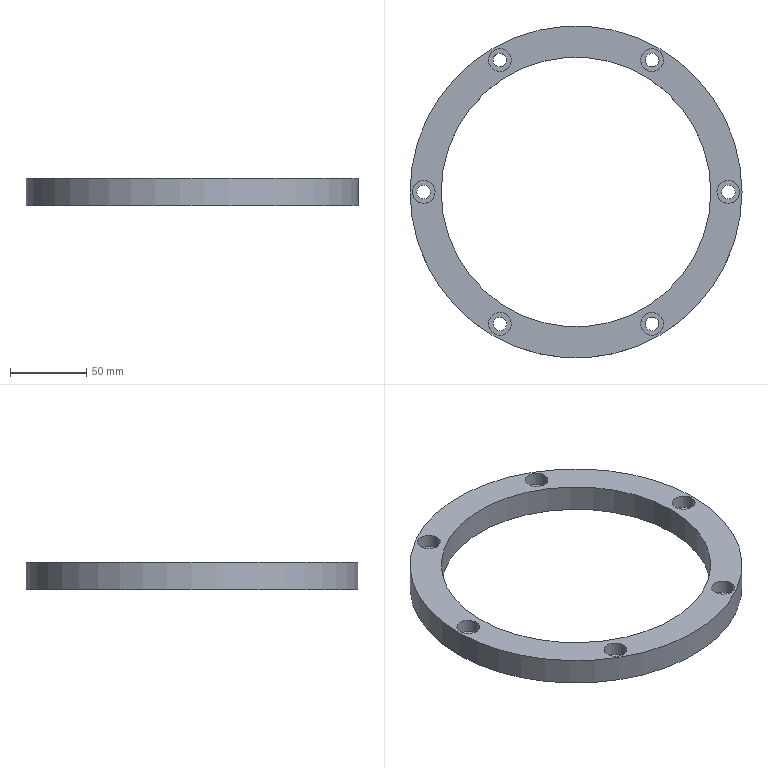Part | NX | 1 solid | 22 faces | box 218 x 218 x 18 mm | volume 215973 mm3 | cylinder 14 | plane 8 | commonest cylinder face diameters 9 x6 15 x6 177 x1 218 x1
STEP:
#1=CARTESIAN_POINT('',(-52.25,-90.5,-18.));
#2=VERTEX_POINT('',#1);
#3=CARTESIAN_POINT('',(-50.,-86.603,-18.));
#4=DIRECTION('',(0.,0.,1.));
#5=DIRECTION('',(-0.5,-0.866,0.));
#6=AXIS2_PLACEMENT_3D('',#3,#4,#5);
#7=CIRCLE('',#6,4.5);
#8=EDGE_CURVE('',#2,#2,#7,.T.);
#9=ORIENTED_EDGE('',*,*,#8,.F.);
#10=EDGE_LOOP('',(#9));
#11=FACE_BOUND('',#10,.T.);
#12=CARTESIAN_POINT('',(-45.5,-86.603,-9.));
#13=VERTEX_POINT('',#12);
#14=CARTESIAN_POINT('',(-50.,-86.603,-9.));
#15=DIRECTION('',(0.,0.,1.));
#16=DIRECTION('',(1.,0.,0.));
#17=AXIS2_PLACEMENT_3D('',#14,#15,#16);
#18=CIRCLE('',#17,4.5);
#19=EDGE_CURVE('',#13,#13,#18,.T.);
#20=ORIENTED_EDGE('',*,*,#19,.T.);
#21=EDGE_LOOP('',(#20));
#22=FACE_BOUND('',#21,.T.);
#23=CARTESIAN_POINT('',(-50.,-86.603,0.));
#24=DIRECTION('',(0.,0.,-1.));
#25=DIRECTION('',(-1.,0.,0.));
#26=AXIS2_PLACEMENT_3D('',#23,#24,#25);
#27=CYLINDRICAL_SURFACE('',#26,4.5);
#28=ADVANCED_FACE('',(#11,#22),#27,.F.);
#29=CARTESIAN_POINT('',(52.25,-90.5,-18.));
#30=VERTEX_POINT('',#29);
#31=CARTESIAN_POINT('',(50.,-86.603,-18.));
#32=DIRECTION('',(0.,0.,1.));
#33=DIRECTION('',(0.5,-0.866,0.));
#34=AXIS2_PLACEMENT_3D('',#31,#32,#33);
#35=CIRCLE('',#34,4.5);
#36=EDGE_CURVE('',#30,#30,#35,.T.);
#37=ORIENTED_EDGE('',*,*,#36,.F.);
#38=EDGE_LOOP('',(#37));
#39=FACE_BOUND('',#38,.T.);
#40=CARTESIAN_POINT('',(54.5,-86.603,-9.));
#41=VERTEX_POINT('',#40);
#42=CARTESIAN_POINT('',(50.,-86.603,-9.));
#43=DIRECTION('',(0.,0.,1.));
#44=DIRECTION('',(1.,0.,0.));
#45=AXIS2_PLACEMENT_3D('',#42,#43,#44);
#46=CIRCLE('',#45,4.5);
#47=EDGE_CURVE('',#41,#41,#46,.T.);
#48=ORIENTED_EDGE('',*,*,#47,.T.);
#49=EDGE_LOOP('',(#48));
#50=FACE_BOUND('',#49,.T.);
#51=CARTESIAN_POINT('',(50.,-86.603,0.));
#52=DIRECTION('',(0.,0.,-1.));
#53=DIRECTION('',(-1.,0.,0.));
#54=AXIS2_PLACEMENT_3D('',#51,#52,#53);
#55=CYLINDRICAL_SURFACE('',#54,4.5);
#56=ADVANCED_FACE('',(#39,#50),#55,.F.);
#57=CARTESIAN_POINT('',(52.25,90.5,-18.));
#58=VERTEX_POINT('',#57);
#59=CARTESIAN_POINT('',(50.,86.603,-18.));
#60=DIRECTION('',(0.,0.,1.));
#61=DIRECTION('',(0.5,0.866,0.));
#62=AXIS2_PLACEMENT_3D('',#59,#60,#61);
#63=CIRCLE('',#62,4.5);
#64=EDGE_CURVE('',#58,#58,#63,.T.);
#65=ORIENTED_EDGE('',*,*,#64,.F.);
#66=EDGE_LOOP('',(#65));
#67=FACE_BOUND('',#66,.T.);
#68=CARTESIAN_POINT('',(54.5,86.603,-9.));
#69=VERTEX_POINT('',#68);
#70=CARTESIAN_POINT('',(50.,86.603,-9.));
#71=DIRECTION('',(0.,0.,1.));
#72=DIRECTION('',(1.,0.,0.));
#73=AXIS2_PLACEMENT_3D('',#70,#71,#72);
#74=CIRCLE('',#73,4.5);
#75=EDGE_CURVE('',#69,#69,#74,.T.);
#76=ORIENTED_EDGE('',*,*,#75,.T.);
#77=EDGE_LOOP('',(#76));
#78=FACE_BOUND('',#77,.T.);
#79=CARTESIAN_POINT('',(50.,86.603,0.));
#80=DIRECTION('',(0.,0.,-1.));
#81=DIRECTION('',(-1.,0.,0.));
#82=AXIS2_PLACEMENT_3D('',#79,#80,#81);
#83=CYLINDRICAL_SURFACE('',#82,4.5);
#84=ADVANCED_FACE('',(#67,#78),#83,.F.);
#85=CARTESIAN_POINT('',(104.5,0.,-18.));
#86=VERTEX_POINT('',#85);
#87=CARTESIAN_POINT('',(100.,0.,-18.));
#88=DIRECTION('',(0.,0.,1.));
#89=DIRECTION('',(1.,0.,0.));
#90=AXIS2_PLACEMENT_3D('',#87,#88,#89);
#91=CIRCLE('',#90,4.5);
#92=EDGE_CURVE('',#86,#86,#91,.T.);
#93=ORIENTED_EDGE('',*,*,#92,.F.);
#94=EDGE_LOOP('',(#93));
#95=FACE_BOUND('',#94,.T.);
#96=CARTESIAN_POINT('',(104.5,0.,-9.));
#97=VERTEX_POINT('',#96);
#98=CARTESIAN_POINT('',(100.,0.,-9.));
#99=DIRECTION('',(0.,0.,1.));
#100=DIRECTION('',(1.,0.,0.));
#101=AXIS2_PLACEMENT_3D('',#98,#99,#100);
#102=CIRCLE('',#101,4.5);
#103=EDGE_CURVE('',#97,#97,#102,.T.);
#104=ORIENTED_EDGE('',*,*,#103,.T.);
#105=EDGE_LOOP('',(#104));
#106=FACE_BOUND('',#105,.T.);
#107=CARTESIAN_POINT('',(100.,0.,0.));
#108=DIRECTION('',(0.,0.,-1.));
#109=DIRECTION('',(-1.,0.,0.));
#110=AXIS2_PLACEMENT_3D('',#107,#108,#109);
#111=CYLINDRICAL_SURFACE('',#110,4.5);
#112=ADVANCED_FACE('',(#95,#106),#111,.F.);
#113=CARTESIAN_POINT('',(-104.5,0.,-18.));
#114=VERTEX_POINT('',#113);
#115=CARTESIAN_POINT('',(-100.,0.,-18.));
#116=DIRECTION('',(0.,0.,1.));
#117=DIRECTION('',(-1.,0.,0.));
#118=AXIS2_PLACEMENT_3D('',#115,#116,#117);
#119=CIRCLE('',#118,4.5);
#120=EDGE_CURVE('',#114,#114,#119,.T.);
#121=ORIENTED_EDGE('',*,*,#120,.F.);
#122=EDGE_LOOP('',(#121));
#123=FACE_BOUND('',#122,.T.);
#124=CARTESIAN_POINT('',(-95.5,0.,-9.));
#125=VERTEX_POINT('',#124);
#126=CARTESIAN_POINT('',(-100.,0.,-9.));
#127=DIRECTION('',(0.,0.,1.));
#128=DIRECTION('',(1.,0.,0.));
#129=AXIS2_PLACEMENT_3D('',#126,#127,#128);
#130=CIRCLE('',#129,4.5);
#131=EDGE_CURVE('',#125,#125,#130,.T.);
#132=ORIENTED_EDGE('',*,*,#131,.T.);
#133=EDGE_LOOP('',(#132));
#134=FACE_BOUND('',#133,.T.);
#135=CARTESIAN_POINT('',(-100.,0.,0.));
#136=DIRECTION('',(0.,0.,-1.));
#137=DIRECTION('',(-1.,0.,0.));
#138=AXIS2_PLACEMENT_3D('',#135,#136,#137);
#139=CYLINDRICAL_SURFACE('',#138,4.5);
#140=ADVANCED_FACE('',(#123,#134),#139,.F.);
#141=CARTESIAN_POINT('',(107.5,0.,0.));
#142=VERTEX_POINT('',#141);
#143=CARTESIAN_POINT('',(100.,0.,0.));
#144=DIRECTION('',(0.,0.,1.));
#145=DIRECTION('',(1.,0.,0.));
#146=AXIS2_PLACEMENT_3D('',#143,#144,#145);
#147=CIRCLE('',#146,7.5);
#148=EDGE_CURVE('',#142,#142,#147,.T.);
#149=ORIENTED_EDGE('',*,*,#148,.F.);
#150=EDGE_LOOP('',(#149));
#151=FACE_BOUND('',#150,.T.);
#152=CARTESIAN_POINT('',(88.5,0.,0.));
#153=VERTEX_POINT('',#152);
#154=CARTESIAN_POINT('',(0.,0.,0.));
#155=DIRECTION('',(0.,0.,1.));
#156=DIRECTION('',(1.,0.,0.));
#157=AXIS2_PLACEMENT_3D('',#154,#155,#156);
#158=CIRCLE('',#157,88.5);
#159=EDGE_CURVE('',#153,#153,#158,.T.);
#160=ORIENTED_EDGE('',*,*,#159,.F.);
#161=EDGE_LOOP('',(#160));
#162=FACE_BOUND('',#161,.T.);
#163=CARTESIAN_POINT('',(109.,0.,0.));
#164=VERTEX_POINT('',#163);
#165=CARTESIAN_POINT('',(0.,0.,0.));
#166=DIRECTION('',(0.,0.,1.));
#167=DIRECTION('',(1.,0.,0.));
#168=AXIS2_PLACEMENT_3D('',#165,#166,#167);
#169=CIRCLE('',#168,109.);
#170=EDGE_CURVE('',#164,#164,#169,.T.);
#171=ORIENTED_EDGE('',*,*,#170,.T.);
#172=EDGE_LOOP('',(#171));
#173=FACE_BOUND('',#172,.T.);
#174=CARTESIAN_POINT('',(53.75,93.098,0.));
#175=VERTEX_POINT('',#174);
#176=CARTESIAN_POINT('',(50.,86.603,0.));
#177=DIRECTION('',(0.,0.,1.));
#178=DIRECTION('',(0.5,0.866,0.));
#179=AXIS2_PLACEMENT_3D('',#176,#177,#178);
#180=CIRCLE('',#179,7.5);
#181=EDGE_CURVE('',#175,#175,#180,.T.);
#182=ORIENTED_EDGE('',*,*,#181,.F.);
#183=EDGE_LOOP('',(#182));
#184=FACE_BOUND('',#183,.T.);
#185=CARTESIAN_POINT('',(53.75,-93.098,0.));
#186=VERTEX_POINT('',#185);
#187=CARTESIAN_POINT('',(50.,-86.603,0.));
#188=DIRECTION('',(0.,0.,1.));
#189=DIRECTION('',(0.5,-0.866,0.));
#190=AXIS2_PLACEMENT_3D('',#187,#188,#189);
#191=CIRCLE('',#190,7.5);
#192=EDGE_CURVE('',#186,#186,#191,.T.);
#193=ORIENTED_EDGE('',*,*,#192,.F.);
#194=EDGE_LOOP('',(#193));
#195=FACE_BOUND('',#194,.T.);
#196=CARTESIAN_POINT('',(-107.5,0.,0.));
#197=VERTEX_POINT('',#196);
#198=CARTESIAN_POINT('',(-100.,0.,0.));
#199=DIRECTION('',(0.,0.,1.));
#200=DIRECTION('',(-1.,0.,0.));
#201=AXIS2_PLACEMENT_3D('',#198,#199,#200);
#202=CIRCLE('',#201,7.5);
#203=EDGE_CURVE('',#197,#197,#202,.T.);
#204=ORIENTED_EDGE('',*,*,#203,.F.);
#205=EDGE_LOOP('',(#204));
#206=FACE_BOUND('',#205,.T.);
#207=CARTESIAN_POINT('',(-53.75,-93.098,0.));
#208=VERTEX_POINT('',#207);
#209=CARTESIAN_POINT('',(-50.,-86.603,0.));
#210=DIRECTION('',(0.,0.,1.));
#211=DIRECTION('',(-0.5,-0.866,0.));
#212=AXIS2_PLACEMENT_3D('',#209,#210,#211);
#213=CIRCLE('',#212,7.5);
#214=EDGE_CURVE('',#208,#208,#213,.T.);
#215=ORIENTED_EDGE('',*,*,#214,.F.);
#216=EDGE_LOOP('',(#215));
#217=FACE_BOUND('',#216,.T.);
#218=CARTESIAN_POINT('',(-53.75,93.098,0.));
#219=VERTEX_POINT('',#218);
#220=CARTESIAN_POINT('',(-50.,86.603,0.));
#221=DIRECTION('',(0.,0.,-1.));
#222=DIRECTION('',(-0.5,0.866,0.));
#223=AXIS2_PLACEMENT_3D('',#220,#221,#222);
#224=CIRCLE('',#223,7.5);
#225=EDGE_CURVE('',#219,#219,#224,.T.);
#226=ORIENTED_EDGE('',*,*,#225,.T.);
#227=EDGE_LOOP('',(#226));
#228=FACE_BOUND('',#227,.T.);
#229=CARTESIAN_POINT('',(50.,0.,0.));
#230=DIRECTION('',(0.,0.,1.));
#231=DIRECTION('',(1.,0.,0.));
#232=AXIS2_PLACEMENT_3D('',#229,#230,#231);
#233=PLANE('',#232);
#234=ADVANCED_FACE('',(#151,#162,#173,#184,#195,#206,#217,#228),#233,.T.);
#235=ORIENTED_EDGE('',*,*,#159,.T.);
#236=EDGE_LOOP('',(#235));
#237=FACE_BOUND('',#236,.T.);
#238=CARTESIAN_POINT('',(88.5,0.,-18.));
#239=VERTEX_POINT('',#238);
#240=CARTESIAN_POINT('',(0.,0.,-18.));
#241=DIRECTION('',(0.,0.,1.));
#242=DIRECTION('',(1.,0.,0.));
#243=AXIS2_PLACEMENT_3D('',#240,#241,#242);
#244=CIRCLE('',#243,88.5);
#245=EDGE_CURVE('',#239,#239,#244,.T.);
#246=ORIENTED_EDGE('',*,*,#245,.F.);
#247=EDGE_LOOP('',(#246));
#248=FACE_BOUND('',#247,.T.);
#249=CARTESIAN_POINT('',(0.,0.,0.));
#250=DIRECTION('',(0.,0.,-1.));
#251=DIRECTION('',(-1.,0.,0.));
#252=AXIS2_PLACEMENT_3D('',#249,#250,#251);
#253=CYLINDRICAL_SURFACE('',#252,88.5);
#254=ADVANCED_FACE('',(#237,#248),#253,.F.);
#255=CARTESIAN_POINT('',(-54.5,86.603,-9.));
#256=VERTEX_POINT('',#255);
#257=CARTESIAN_POINT('',(-50.,86.603,-9.));
#258=DIRECTION('',(0.,0.,-1.));
#259=DIRECTION('',(-1.,0.,0.));
#260=AXIS2_PLACEMENT_3D('',#257,#258,#259);
#261=CIRCLE('',#260,4.5);
#262=EDGE_CURVE('',#256,#256,#261,.T.);
#263=ORIENTED_EDGE('',*,*,#262,.F.);
#264=EDGE_LOOP('',(#263));
#265=FACE_BOUND('',#264,.T.);
#266=CARTESIAN_POINT('',(-52.25,90.5,-18.));
#267=VERTEX_POINT('',#266);
#268=CARTESIAN_POINT('',(-50.,86.603,-18.));
#269=DIRECTION('',(0.,0.,1.));
#270=DIRECTION('',(-0.5,0.866,0.));
#271=AXIS2_PLACEMENT_3D('',#268,#269,#270);
#272=CIRCLE('',#271,4.5);
#273=EDGE_CURVE('',#267,#267,#272,.T.);
#274=ORIENTED_EDGE('',*,*,#273,.F.);
#275=EDGE_LOOP('',(#274));
#276=FACE_BOUND('',#275,.T.);
#277=CARTESIAN_POINT('',(-50.,86.603,0.));
#278=DIRECTION('',(0.,0.,-1.));
#279=DIRECTION('',(-1.,0.,0.));
#280=AXIS2_PLACEMENT_3D('',#277,#278,#279);
#281=CYLINDRICAL_SURFACE('',#280,4.5);
#282=ADVANCED_FACE('',(#265,#276),#281,.F.);
#283=ORIENTED_EDGE('',*,*,#170,.F.);
#284=EDGE_LOOP('',(#283));
#285=FACE_BOUND('',#284,.T.);
#286=CARTESIAN_POINT('',(109.,0.,-18.));
#287=VERTEX_POINT('',#286);
#288=CARTESIAN_POINT('',(0.,0.,-18.));
#289=DIRECTION('',(0.,0.,1.));
#290=DIRECTION('',(1.,0.,0.));
#291=AXIS2_PLACEMENT_3D('',#288,#289,#290);
#292=CIRCLE('',#291,109.);
#293=EDGE_CURVE('',#287,#287,#292,.T.);
#294=ORIENTED_EDGE('',*,*,#293,.T.);
#295=EDGE_LOOP('',(#294));
#296=FACE_BOUND('',#295,.T.);
#297=CARTESIAN_POINT('',(0.,0.,0.));
#298=DIRECTION('',(0.,0.,-1.));
#299=DIRECTION('',(-1.,0.,0.));
#300=AXIS2_PLACEMENT_3D('',#297,#298,#299);
#301=CYLINDRICAL_SURFACE('',#300,109.);
#302=ADVANCED_FACE('',(#285,#296),#301,.T.);
#303=ORIENTED_EDGE('',*,*,#293,.F.);
#304=EDGE_LOOP('',(#303));
#305=FACE_BOUND('',#304,.T.);
#306=ORIENTED_EDGE('',*,*,#92,.T.);
#307=EDGE_LOOP('',(#306));
#308=FACE_BOUND('',#307,.T.);
#309=ORIENTED_EDGE('',*,*,#64,.T.);
#310=EDGE_LOOP('',(#309));
#311=FACE_BOUND('',#310,.T.);
#312=ORIENTED_EDGE('',*,*,#36,.T.);
#313=EDGE_LOOP('',(#312));
#314=FACE_BOUND('',#313,.T.);
#315=ORIENTED_EDGE('',*,*,#273,.T.);
#316=EDGE_LOOP('',(#315));
#317=FACE_BOUND('',#316,.T.);
#318=ORIENTED_EDGE('',*,*,#8,.T.);
#319=EDGE_LOOP('',(#318));
#320=FACE_BOUND('',#319,.T.);
#321=ORIENTED_EDGE('',*,*,#245,.T.);
#322=EDGE_LOOP('',(#321));
#323=FACE_BOUND('',#322,.T.);
#324=ORIENTED_EDGE('',*,*,#120,.T.);
#325=EDGE_LOOP('',(#324));
#326=FACE_BOUND('',#325,.T.);
#327=CARTESIAN_POINT('',(50.,0.,-18.));
#328=DIRECTION('',(0.,0.,1.));
#329=DIRECTION('',(1.,0.,0.));
#330=AXIS2_PLACEMENT_3D('',#327,#328,#329);
#331=PLANE('',#330);
#332=ADVANCED_FACE('',(#305,#308,#311,#314,#317,#320,#323,#326),#331,.F.);
#333=ORIENTED_EDGE('',*,*,#181,.T.);
#334=EDGE_LOOP('',(#333));
#335=FACE_BOUND('',#334,.T.);
#336=CARTESIAN_POINT('',(53.75,93.098,-9.));
#337=VERTEX_POINT('',#336);
#338=CARTESIAN_POINT('',(50.,86.603,-9.));
#339=DIRECTION('',(0.,0.,1.));
#340=DIRECTION('',(0.5,0.866,0.));
#341=AXIS2_PLACEMENT_3D('',#338,#339,#340);
#342=CIRCLE('',#341,7.5);
#343=EDGE_CURVE('',#337,#337,#342,.F.);
#344=ORIENTED_EDGE('',*,*,#343,.T.);
#345=EDGE_LOOP('',(#344));
#346=FACE_BOUND('',#345,.T.);
#347=CARTESIAN_POINT('',(50.,86.603,0.));
#348=DIRECTION('',(0.,0.,-1.));
#349=DIRECTION('',(-1.,0.,0.));
#350=AXIS2_PLACEMENT_3D('',#347,#348,#349);
#351=CYLINDRICAL_SURFACE('',#350,7.5);
#352=ADVANCED_FACE('',(#335,#346),#351,.F.);
#353=ORIENTED_EDGE('',*,*,#75,.F.);
#354=EDGE_LOOP('',(#353));
#355=FACE_BOUND('',#354,.T.);
#356=ORIENTED_EDGE('',*,*,#343,.F.);
#357=EDGE_LOOP('',(#356));
#358=FACE_BOUND('',#357,.T.);
#359=CARTESIAN_POINT('',(50.,86.603,-9.));
#360=DIRECTION('',(0.,0.,1.));
#361=DIRECTION('',(1.,0.,0.));
#362=AXIS2_PLACEMENT_3D('',#359,#360,#361);
#363=PLANE('',#362);
#364=ADVANCED_FACE('',(#355,#358),#363,.T.);
#365=ORIENTED_EDGE('',*,*,#192,.T.);
#366=EDGE_LOOP('',(#365));
#367=FACE_BOUND('',#366,.T.);
#368=CARTESIAN_POINT('',(53.75,-93.098,-9.));
#369=VERTEX_POINT('',#368);
#370=CARTESIAN_POINT('',(50.,-86.603,-9.));
#371=DIRECTION('',(0.,0.,1.));
#372=DIRECTION('',(0.5,-0.866,0.));
#373=AXIS2_PLACEMENT_3D('',#370,#371,#372);
#374=CIRCLE('',#373,7.5);
#375=EDGE_CURVE('',#369,#369,#374,.F.);
#376=ORIENTED_EDGE('',*,*,#375,.T.);
#377=EDGE_LOOP('',(#376));
#378=FACE_BOUND('',#377,.T.);
#379=CARTESIAN_POINT('',(50.,-86.603,0.));
#380=DIRECTION('',(0.,0.,-1.));
#381=DIRECTION('',(-1.,0.,0.));
#382=AXIS2_PLACEMENT_3D('',#379,#380,#381);
#383=CYLINDRICAL_SURFACE('',#382,7.5);
#384=ADVANCED_FACE('',(#367,#378),#383,.F.);
#385=ORIENTED_EDGE('',*,*,#47,.F.);
#386=EDGE_LOOP('',(#385));
#387=FACE_BOUND('',#386,.T.);
#388=ORIENTED_EDGE('',*,*,#375,.F.);
#389=EDGE_LOOP('',(#388));
#390=FACE_BOUND('',#389,.T.);
#391=CARTESIAN_POINT('',(50.,-86.603,-9.));
#392=DIRECTION('',(0.,0.,1.));
#393=DIRECTION('',(1.,0.,0.));
#394=AXIS2_PLACEMENT_3D('',#391,#392,#393);
#395=PLANE('',#394);
#396=ADVANCED_FACE('',(#387,#390),#395,.T.);
#397=ORIENTED_EDGE('',*,*,#203,.T.);
#398=EDGE_LOOP('',(#397));
#399=FACE_BOUND('',#398,.T.);
#400=CARTESIAN_POINT('',(-107.5,0.,-9.));
#401=VERTEX_POINT('',#400);
#402=CARTESIAN_POINT('',(-100.,0.,-9.));
#403=DIRECTION('',(0.,0.,1.));
#404=DIRECTION('',(-1.,0.,0.));
#405=AXIS2_PLACEMENT_3D('',#402,#403,#404);
#406=CIRCLE('',#405,7.5);
#407=EDGE_CURVE('',#401,#401,#406,.F.);
#408=ORIENTED_EDGE('',*,*,#407,.T.);
#409=EDGE_LOOP('',(#408));
#410=FACE_BOUND('',#409,.T.);
#411=CARTESIAN_POINT('',(-100.,0.,0.));
#412=DIRECTION('',(0.,0.,-1.));
#413=DIRECTION('',(-1.,0.,0.));
#414=AXIS2_PLACEMENT_3D('',#411,#412,#413);
#415=CYLINDRICAL_SURFACE('',#414,7.5);
#416=ADVANCED_FACE('',(#399,#410),#415,.F.);
#417=ORIENTED_EDGE('',*,*,#131,.F.);
#418=EDGE_LOOP('',(#417));
#419=FACE_BOUND('',#418,.T.);
#420=ORIENTED_EDGE('',*,*,#407,.F.);
#421=EDGE_LOOP('',(#420));
#422=FACE_BOUND('',#421,.T.);
#423=CARTESIAN_POINT('',(-100.,0.,-9.));
#424=DIRECTION('',(0.,0.,1.));
#425=DIRECTION('',(1.,0.,0.));
#426=AXIS2_PLACEMENT_3D('',#423,#424,#425);
#427=PLANE('',#426);
#428=ADVANCED_FACE('',(#419,#422),#427,.T.);
#429=ORIENTED_EDGE('',*,*,#214,.T.);
#430=EDGE_LOOP('',(#429));
#431=FACE_BOUND('',#430,.T.);
#432=CARTESIAN_POINT('',(-53.75,-93.098,-9.));
#433=VERTEX_POINT('',#432);
#434=CARTESIAN_POINT('',(-50.,-86.603,-9.));
#435=DIRECTION('',(0.,0.,1.));
#436=DIRECTION('',(-0.5,-0.866,0.));
#437=AXIS2_PLACEMENT_3D('',#434,#435,#436);
#438=CIRCLE('',#437,7.5);
#439=EDGE_CURVE('',#433,#433,#438,.F.);
#440=ORIENTED_EDGE('',*,*,#439,.T.);
#441=EDGE_LOOP('',(#440));
#442=FACE_BOUND('',#441,.T.);
#443=CARTESIAN_POINT('',(-50.,-86.603,0.));
#444=DIRECTION('',(0.,0.,-1.));
#445=DIRECTION('',(-1.,0.,0.));
#446=AXIS2_PLACEMENT_3D('',#443,#444,#445);
#447=CYLINDRICAL_SURFACE('',#446,7.5);
#448=ADVANCED_FACE('',(#431,#442),#447,.F.);
#449=ORIENTED_EDGE('',*,*,#19,.F.);
#450=EDGE_LOOP('',(#449));
#451=FACE_BOUND('',#450,.T.);
#452=ORIENTED_EDGE('',*,*,#439,.F.);
#453=EDGE_LOOP('',(#452));
#454=FACE_BOUND('',#453,.T.);
#455=CARTESIAN_POINT('',(-50.,-86.603,-9.));
#456=DIRECTION('',(0.,0.,1.));
#457=DIRECTION('',(1.,0.,0.));
#458=AXIS2_PLACEMENT_3D('',#455,#456,#457);
#459=PLANE('',#458);
#460=ADVANCED_FACE('',(#451,#454),#459,.T.);
#461=ORIENTED_EDGE('',*,*,#225,.F.);
#462=EDGE_LOOP('',(#461));
#463=FACE_BOUND('',#462,.T.);
#464=CARTESIAN_POINT('',(-53.75,93.098,-9.));
#465=VERTEX_POINT('',#464);
#466=CARTESIAN_POINT('',(-50.,86.603,-9.));
#467=DIRECTION('',(0.,0.,-1.));
#468=DIRECTION('',(-0.5,0.866,0.));
#469=AXIS2_PLACEMENT_3D('',#466,#467,#468);
#470=CIRCLE('',#469,7.5);
#471=EDGE_CURVE('',#465,#465,#470,.F.);
#472=ORIENTED_EDGE('',*,*,#471,.F.);
#473=EDGE_LOOP('',(#472));
#474=FACE_BOUND('',#473,.T.);
#475=CARTESIAN_POINT('',(-50.,86.603,0.));
#476=DIRECTION('',(0.,0.,-1.));
#477=DIRECTION('',(-1.,0.,0.));
#478=AXIS2_PLACEMENT_3D('',#475,#476,#477);
#479=CYLINDRICAL_SURFACE('',#478,7.5);
#480=ADVANCED_FACE('',(#463,#474),#479,.F.);
#481=ORIENTED_EDGE('',*,*,#262,.T.);
#482=EDGE_LOOP('',(#481));
#483=FACE_BOUND('',#482,.T.);
#484=ORIENTED_EDGE('',*,*,#471,.T.);
#485=EDGE_LOOP('',(#484));
#486=FACE_BOUND('',#485,.T.);
#487=CARTESIAN_POINT('',(-50.,86.603,-9.));
#488=DIRECTION('',(0.,0.,-1.));
#489=DIRECTION('',(-1.,0.,0.));
#490=AXIS2_PLACEMENT_3D('',#487,#488,#489);
#491=PLANE('',#490);
#492=ADVANCED_FACE('',(#483,#486),#491,.F.);
#493=ORIENTED_EDGE('',*,*,#148,.T.);
#494=EDGE_LOOP('',(#493));
#495=FACE_BOUND('',#494,.T.);
#496=CARTESIAN_POINT('',(107.5,0.,-9.));
#497=VERTEX_POINT('',#496);
#498=CARTESIAN_POINT('',(100.,0.,-9.));
#499=DIRECTION('',(0.,0.,1.));
#500=DIRECTION('',(1.,0.,0.));
#501=AXIS2_PLACEMENT_3D('',#498,#499,#500);
#502=CIRCLE('',#501,7.5);
#503=EDGE_CURVE('',#497,#497,#502,.F.);
#504=ORIENTED_EDGE('',*,*,#503,.T.);
#505=EDGE_LOOP('',(#504));
#506=FACE_BOUND('',#505,.T.);
#507=CARTESIAN_POINT('',(100.,0.,0.));
#508=DIRECTION('',(0.,0.,-1.));
#509=DIRECTION('',(-1.,0.,0.));
#510=AXIS2_PLACEMENT_3D('',#507,#508,#509);
#511=CYLINDRICAL_SURFACE('',#510,7.5);
#512=ADVANCED_FACE('',(#495,#506),#511,.F.);
#513=ORIENTED_EDGE('',*,*,#103,.F.);
#514=EDGE_LOOP('',(#513));
#515=FACE_BOUND('',#514,.T.);
#516=ORIENTED_EDGE('',*,*,#503,.F.);
#517=EDGE_LOOP('',(#516));
#518=FACE_BOUND('',#517,.T.);
#519=CARTESIAN_POINT('',(100.,0.,-9.));
#520=DIRECTION('',(0.,0.,1.));
#521=DIRECTION('',(1.,0.,0.));
#522=AXIS2_PLACEMENT_3D('',#519,#520,#521);
#523=PLANE('',#522);
#524=ADVANCED_FACE('',(#515,#518),#523,.T.);
#525=CLOSED_SHELL('',(#28,#56,#84,#112,#140,#234,#254,#282,#302,#332,#352,#364,#384,#396,#416,#428,#448,#460,#480,#492,#512,#524));
#526=MANIFOLD_SOLID_BREP('',#525);
#527=(LENGTH_UNIT()NAMED_UNIT(*)SI_UNIT(.MILLI.,.METRE.));
#528=UNCERTAINTY_MEASURE_WITH_UNIT(LENGTH_MEASURE(0.00001),#527,'','');
#529=(NAMED_UNIT(*)PLANE_ANGLE_UNIT()SI_UNIT($,.RADIAN.));
#530=(NAMED_UNIT(*)SI_UNIT($,.STERADIAN.)SOLID_ANGLE_UNIT());
#531=(GEOMETRIC_REPRESENTATION_CONTEXT(3)GLOBAL_UNCERTAINTY_ASSIGNED_CONTEXT((#528))GLOBAL_UNIT_ASSIGNED_CONTEXT((#527,#529,#530))REPRESENTATION_CONTEXT('',''));
#532=ADVANCED_BREP_SHAPE_REPRESENTATION('',(#526),#531);